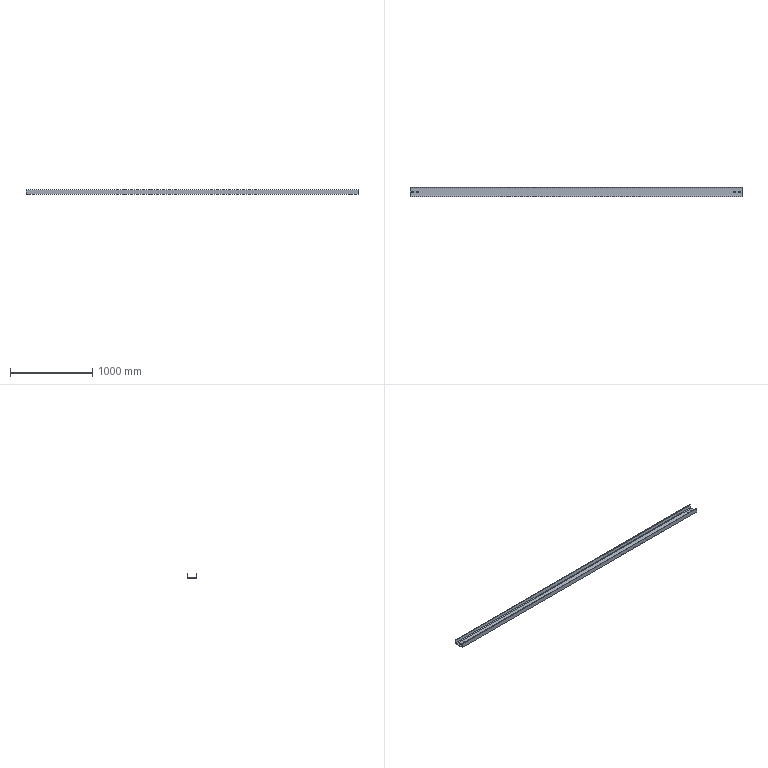Part | STEP file | E3-中转釜连接梁3_Default<As Machined> | 1 solid | 22 faces | box 4030 x 120 x 53 mm | volume 6181162 mm3 | cylinder 12 | plane 10 | commonest cylinder face diameters 19 x8 9 x2 18 x2